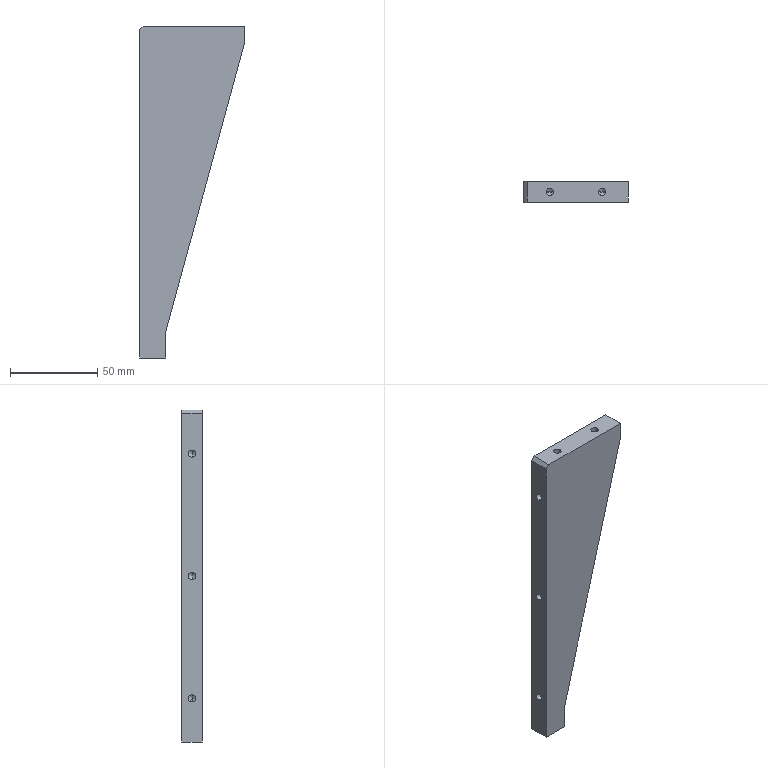Part | STEP file | PN_0034 | 1 solid | 29 faces | box 60 x 12 x 190 mm | volume 83127 mm3 | cylinder 10 | cone 10 | plane 9 | commonest cylinder face diameters 4.2 x10